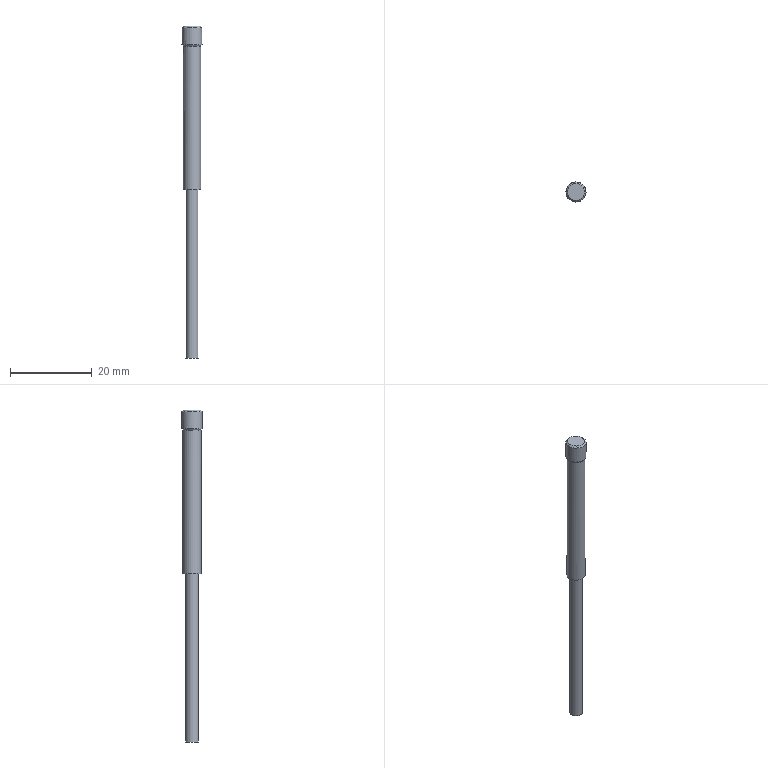Part | NX | features APJEL25-80-P20.00-W16.17_1 2 | 1 solid | 8 faces | box 4.9 x 4.9 x 81 mm | volume 933.916 mm3 | cylinder 3 | plane 3 | spline 1 | cone 1 | commonest cylinder face diameters 3.1 x1 4.4 x1 4.9 x1